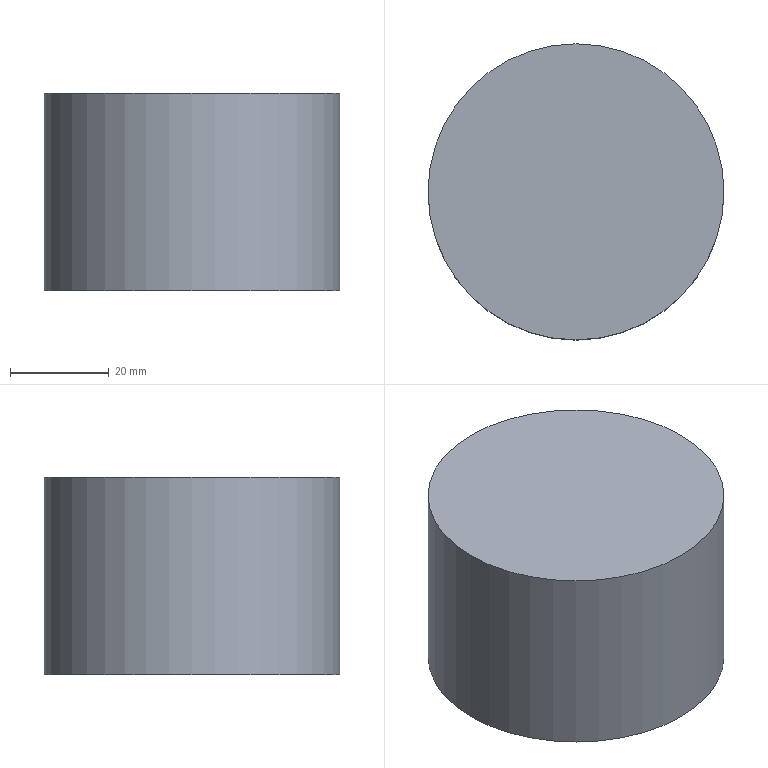Part | NX | features solid 2 | 1 solid | 3 faces | box 60 x 60 x 40 mm | volume 113097 mm3 | plane 2 | cylinder 1 | commonest cylinder face diameters 60 x1
STEP:
#1=CARTESIAN_POINT('',(-1335.,710.,-90.));
#2=VERTEX_POINT('',#1);
#3=CARTESIAN_POINT('',(-1305.,710.,-90.));
#4=DIRECTION('',(0.,0.,-1.));
#5=DIRECTION('',(-1.,0.,0.));
#6=AXIS2_PLACEMENT_3D('',#3,#4,#5);
#7=CIRCLE('',#6,30.);
#8=EDGE_CURVE('',#2,#2,#7,.F.);
#9=ORIENTED_EDGE('',*,*,#8,.F.);
#10=EDGE_LOOP('',(#9));
#11=FACE_BOUND('',#10,.T.);
#12=CARTESIAN_POINT('',(-1335.,710.,-130.));
#13=VERTEX_POINT('',#12);
#14=CARTESIAN_POINT('',(-1305.,710.,-130.));
#15=DIRECTION('',(0.,0.,-1.));
#16=DIRECTION('',(-1.,0.,0.));
#17=AXIS2_PLACEMENT_3D('',#14,#15,#16);
#18=CIRCLE('',#17,30.);
#19=EDGE_CURVE('',#13,#13,#18,.F.);
#20=ORIENTED_EDGE('',*,*,#19,.T.);
#21=EDGE_LOOP('',(#20));
#22=FACE_BOUND('',#21,.T.);
#23=CARTESIAN_POINT('',(-1305.,710.,-110.));
#24=DIRECTION('',(0.,0.,-1.));
#25=DIRECTION('',(1.,0.,0.));
#26=AXIS2_PLACEMENT_3D('',#23,#24,#25);
#27=CYLINDRICAL_SURFACE('',#26,30.);
#28=ADVANCED_FACE('',(#11,#22),#27,.T.);
#29=ORIENTED_EDGE('',*,*,#8,.T.);
#30=EDGE_LOOP('',(#29));
#31=FACE_BOUND('',#30,.T.);
#32=CARTESIAN_POINT('',(-1305.,710.,-90.));
#33=DIRECTION('',(0.,0.,1.));
#34=DIRECTION('',(-1.,0.,0.));
#35=AXIS2_PLACEMENT_3D('',#32,#33,#34);
#36=PLANE('',#35);
#37=ADVANCED_FACE('',(#31),#36,.T.);
#38=ORIENTED_EDGE('',*,*,#19,.F.);
#39=EDGE_LOOP('',(#38));
#40=FACE_BOUND('',#39,.T.);
#41=CARTESIAN_POINT('',(-1305.,710.,-130.));
#42=DIRECTION('',(0.,0.,1.));
#43=DIRECTION('',(-1.,0.,0.));
#44=AXIS2_PLACEMENT_3D('',#41,#42,#43);
#45=PLANE('',#44);
#46=ADVANCED_FACE('',(#40),#45,.F.);
#47=CLOSED_SHELL('',(#28,#37,#46));
#48=MANIFOLD_SOLID_BREP('',#47);
#49=(LENGTH_UNIT()NAMED_UNIT(*)SI_UNIT(.MILLI.,.METRE.));
#50=UNCERTAINTY_MEASURE_WITH_UNIT(LENGTH_MEASURE(0.00001),#49,'','');
#51=(NAMED_UNIT(*)PLANE_ANGLE_UNIT()SI_UNIT($,.RADIAN.));
#52=(NAMED_UNIT(*)SI_UNIT($,.STERADIAN.)SOLID_ANGLE_UNIT());
#53=(GEOMETRIC_REPRESENTATION_CONTEXT(3)GLOBAL_UNCERTAINTY_ASSIGNED_CONTEXT((#50))GLOBAL_UNIT_ASSIGNED_CONTEXT((#49,#51,#52))REPRESENTATION_CONTEXT('',''));
#54=ADVANCED_BREP_SHAPE_REPRESENTATION('',(#48),#53);